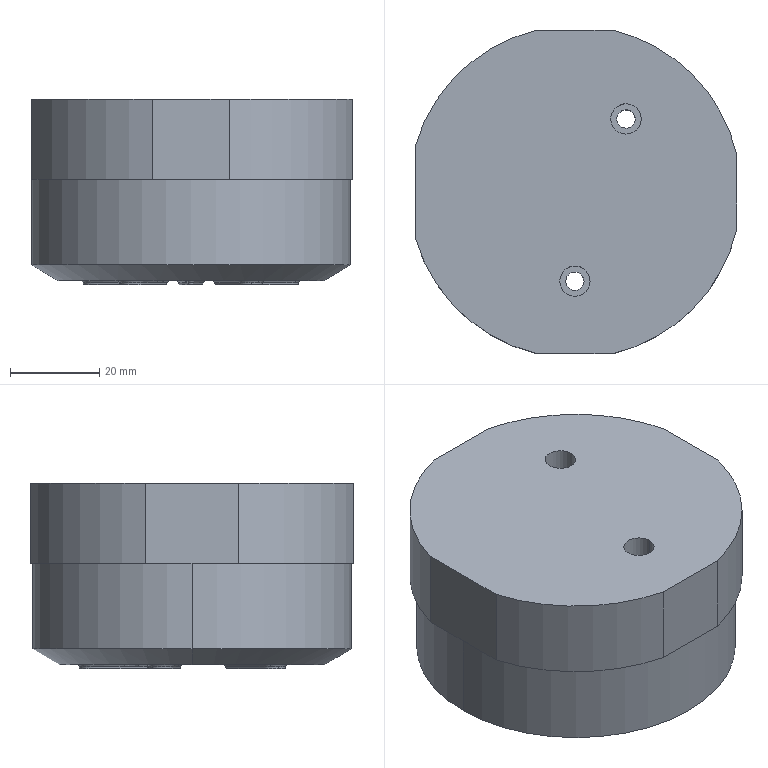Part | SolidWorks | features BaseBody 1 | 1 solid | 50 faces | box 72 x 72.5 x 41.7 mm | volume 164977 mm3 | spline 20 | cylinder 14 | plane 14 | cone 2 | commonest cylinder face diameters 4.101 x4 6.805 x4 74.5 x4 71.5 x2